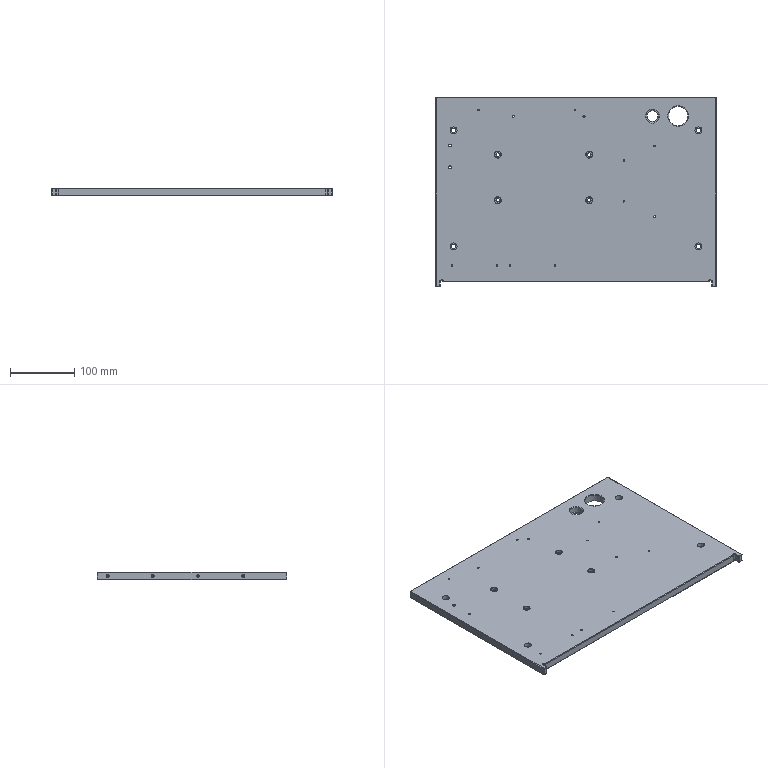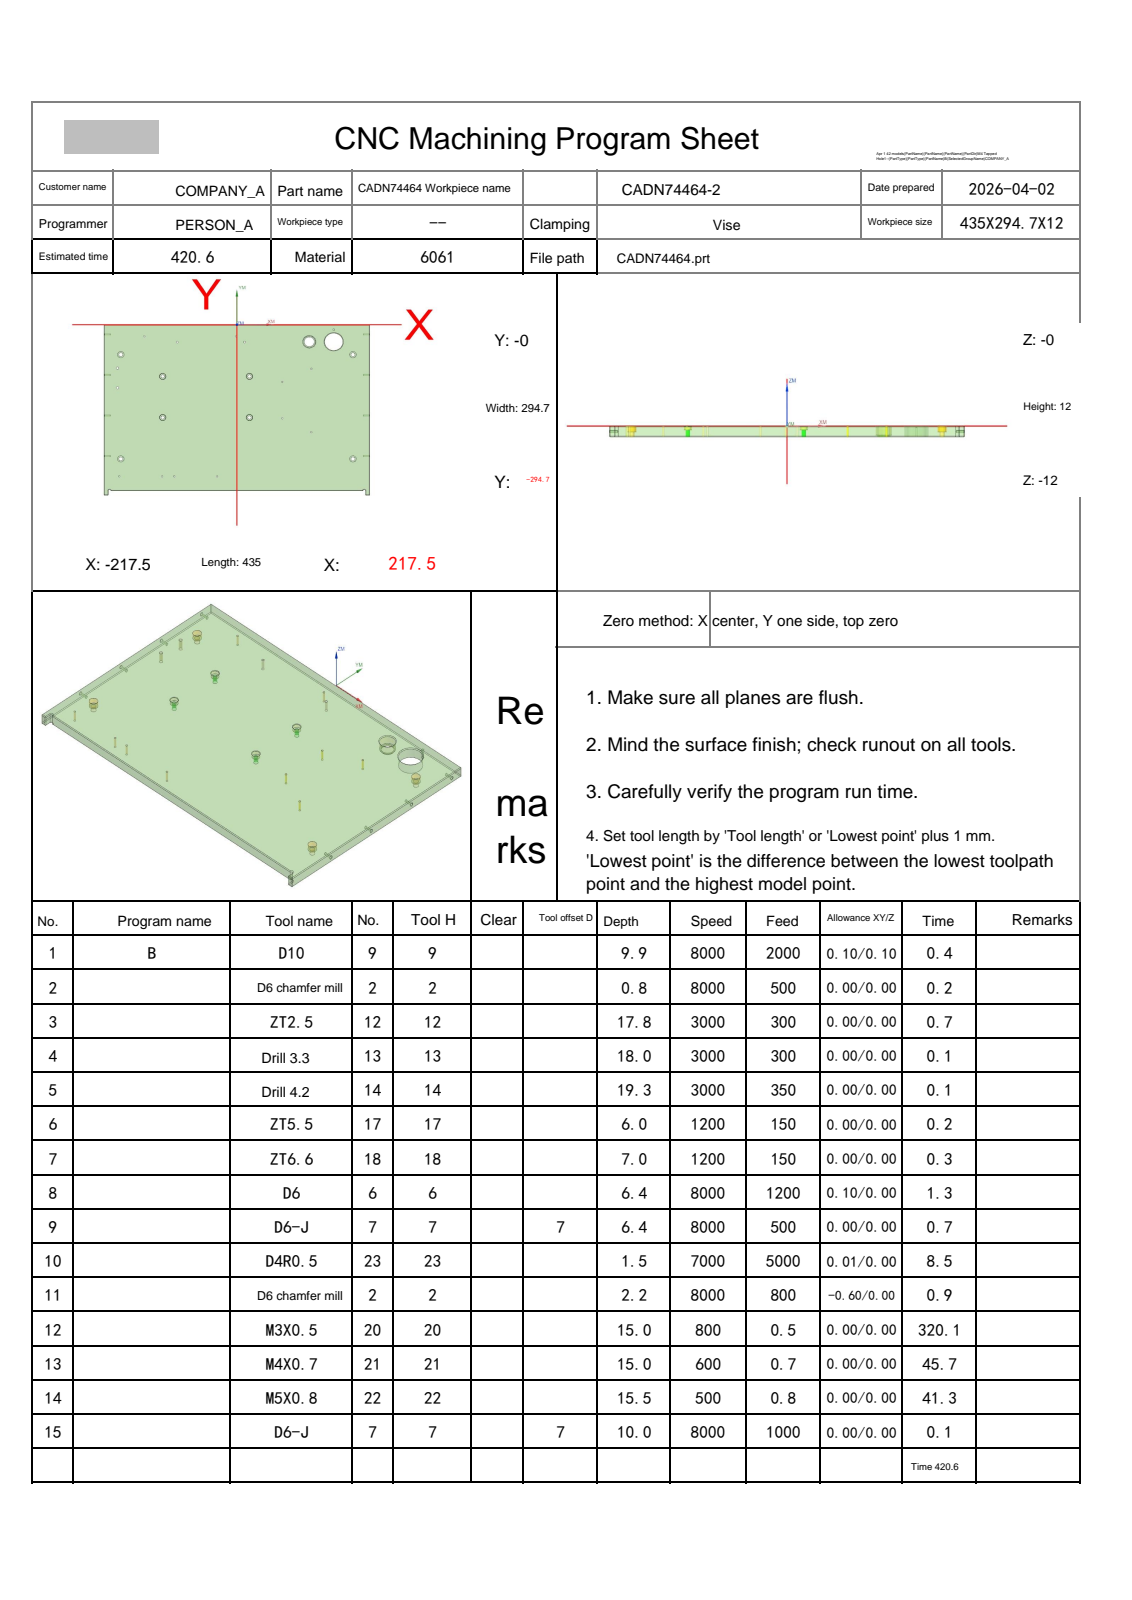NC program | NX | posted by the shop | part box 435 x 294.7 x 12 mm
Lines 33526 to 33933 of 33933:
N11 T02 M06
(D6 chamfer mill  D=6. R=0. H=02 ce=0.00 di=0.00)
G00 G90 G54 X-151.5 Y-20. M03 S8000
G43 H02 Z20.
M08
G98 G81 X-151.5 Y-20. Z-1.75 R3. F500.
X-1.5
X74.218 Y-98.649
X121.901 Y-76.021
Y-185.521
X74.218 Y-161.649
X-32.5 Y-261.7
X-102.5
X-122.5
X-192.5
G80
G00 Z20.
G00 G90 X-97.5 Y-30. M03 S8000
Z20.
G98 G81 X-97.5 Y-30. Z-2.2 R3. F500.
X12.5
G80
G00 Z20.
G00 G90 X-195.593 Y-108.306 M03 S8000
Z20.
Z-.5
G01 Z-1. F500.
X-195.7 Y-107.5
G03 X-197.2 Y-109. I0.0 J-1.5
X-195.5 Y-110.7 I1.7 J0.0
X-193.8 Y-109. I0.0 J1.7
X-195.5 Y-107.3 I-1.7 J0.0
X-197.2 Y-109. I0.0 J-1.7
X-195.7 Y-110.5 I1.5 J0.0
G01 X-195.593 Y-109.694
Z-.5
G00 Z20.
Y-74.306
Z-.5
G01 Z-1.
X-195.7 Y-73.5
G03 X-197.2 Y-75. I0.0 J-1.5
X-195.5 Y-76.7 I1.7 J0.0
X-193.8 Y-75. I0.0 J1.7
X-195.5 Y-73.3 I-1.7 J0.0
X-197.2 Y-75. I0.0 J-1.7
X-195.7 Y-76.5 I1.5 J0.0
G01 X-195.593 Y-75.694
Z-.5
G00 Z20.
G00 G90 X-125.117 Y-161.779 M03 S8000
Z20.
Z2.5
G01 X-124.98 Y-162.081 Z2.379 F800.
X-124.765 Y-162.447 Z2.225
X-124.512 Y-162.789 Z2.07
X-124.225 Y-163.102 Z1.916
X-123.906 Y-163.382 Z1.761
X-123.559 Y-163.627 Z1.606
X-123.291 Y-163.782 Z1.494
X-122.905 Y-163.96 Z1.339
X-122.503 Y-164.096 Z1.184
X-122.088 Y-164.188 Z1.03
X-121.666 Y-164.237 Z.875
X-121.241 Y-164.24 Z.721
X-120.819 Y-164.198 Z.566
X-120.403 Y-164.111 Z.412
X-119.999 Y-163.981 Z.257
X-119.61 Y-163.809 Z.102
X-119.243 Y-163.596 Z-.052
X-118.899 Y-163.346 Z-.207
X-118.584 Y-163.061 Z-.361
X-118.302 Y-162.744 Z-.516
X-118.054 Y-162.399 Z-.671
X-117.844 Y-162.03 Z-.825
X-117.675 Y-161.64 Z-.98
X-117.548 Y-161.235 Z-1.134
X-117.464 Y-160.819 Z-1.289
X-117.425 Y-160.396 Z-1.444
Y-160.241 Z-1.5
G03 X-121.425 Y-156.241 I-4. J0.0
X-125.425 Y-160.241 I0.0 J-4.
X-121.425 Y-164.241 I4. J0.0
X-117.425 Y-160.241 I0.0 J4.
X-117.456 Y-159.742 I-4. J0.0
G01 Z1.
G00 Z20.
X-125.117 Y-90.779
Z2.5
G01 X-124.98 Y-91.081 Z2.379
X-124.765 Y-91.447 Z2.225
X-124.512 Y-91.789 Z2.07
X-124.225 Y-92.102 Z1.916
X-123.906 Y-92.382 Z1.761
X-123.559 Y-92.627 Z1.606
X-123.291 Y-92.782 Z1.494
X-122.905 Y-92.96 Z1.339
X-122.503 Y-93.096 Z1.184
X-122.088 Y-93.188 Z1.03
X-121.666 Y-93.237 Z.875
X-121.241 Y-93.24 Z.721
X-120.819 Y-93.198 Z.566
X-120.403 Y-93.111 Z.412
X-119.999 Y-92.981 Z.257
X-119.61 Y-92.809 Z.102
X-119.243 Y-92.596 Z-.052
X-118.899 Y-92.346 Z-.207
X-118.584 Y-92.061 Z-.361
X-118.302 Y-91.744 Z-.516
X-118.054 Y-91.399 Z-.671
X-117.844 Y-91.03 Z-.825
X-117.675 Y-90.64 Z-.98
X-117.548 Y-90.235 Z-1.134
X-117.464 Y-89.819 Z-1.289
X-117.425 Y-89.396 Z-1.444
Y-89.241 Z-1.5
G03 X-121.425 Y-85.241 I-4. J0.0
X-125.425 Y-89.241 I0.0 J-4.
X-121.425 Y-93.241 I4. J0.0
X-117.425 Y-89.241 I0.0 J4.
X-117.456 Y-88.742 I-4. J0.0
G01 Z1.
G00 Z20.
X16.883 Y-90.779
Z2.5
G01 X17.02 Y-91.081 Z2.379
X17.235 Y-91.447 Z2.225
X17.488 Y-91.789 Z2.07
X17.775 Y-92.102 Z1.916
X18.094 Y-92.382 Z1.761
X18.441 Y-92.627 Z1.606
X18.709 Y-92.782 Z1.494
X19.095 Y-92.96 Z1.339
X19.497 Y-93.096 Z1.184
X19.912 Y-93.188 Z1.03
X20.334 Y-93.237 Z.875
X20.759 Y-93.24 Z.721
X21.181 Y-93.198 Z.566
X21.597 Y-93.111 Z.412
X22.001 Y-92.981 Z.257
X22.39 Y-92.809 Z.102
X22.757 Y-92.596 Z-.052
X23.101 Y-92.346 Z-.207
X23.416 Y-92.061 Z-.361
X23.698 Y-91.744 Z-.516
X23.946 Y-91.399 Z-.671
X24.156 Y-91.03 Z-.825
X24.325 Y-90.64 Z-.98
X24.452 Y-90.235 Z-1.134
X24.536 Y-89.819 Z-1.289
X24.575 Y-89.396 Z-1.444
Y-89.241 Z-1.5
G03 X20.575 Y-85.241 I-4. J0.0
X16.575 Y-89.241 I0.0 J-4.
X20.575 Y-93.241 I4. J0.0
X24.575 Y-89.241 I0.0 J4.
X24.544 Y-88.742 I-4. J0.0
G01 Z1.
G00 Z20.
X16.883 Y-161.779
Z2.5
G01 X17.02 Y-162.081 Z2.379
X17.235 Y-162.447 Z2.225
X17.488 Y-162.789 Z2.07
X17.775 Y-163.102 Z1.916
X18.094 Y-163.382 Z1.761
X18.441 Y-163.627 Z1.606
X18.709 Y-163.782 Z1.494
X19.095 Y-163.96 Z1.339
X19.497 Y-164.096 Z1.184
X19.912 Y-164.188 Z1.03
X20.334 Y-164.237 Z.875
X20.759 Y-164.24 Z.721
X21.181 Y-164.198 Z.566
X21.597 Y-164.111 Z.412
X22.001 Y-163.981 Z.257
X22.39 Y-163.809 Z.102
X22.757 Y-163.596 Z-.052
X23.101 Y-163.346 Z-.207
X23.416 Y-163.061 Z-.361
X23.698 Y-162.744 Z-.516
X23.946 Y-162.399 Z-.671
X24.156 Y-162.03 Z-.825
X24.325 Y-161.64 Z-.98
X24.452 Y-161.235 Z-1.134
X24.536 Y-160.819 Z-1.289
X24.575 Y-160.396 Z-1.444
Y-160.241 Z-1.5
G03 X20.575 Y-156.241 I-4. J0.0
X16.575 Y-160.241 I0.0 J-4.
X20.575 Y-164.241 I4. J0.0
X24.575 Y-160.241 I0.0 J4.
X24.544 Y-159.742 I-4. J0.0
G01 Z1.
G00 Z20.
G00 G90 X187.991 Y-236.053 M03 S8000
Z20.
Z2.5
G01 X188.166 Y-236.135 Z2.43 F800.
X188.601 Y-236.291 Z2.261
X189.05 Y-236.404 Z2.093
X189.507 Y-236.474 Z1.925
X189.969 Y-236.499 Z1.756
X190.431 Y-236.48 Z1.588
X190.89 Y-236.416 Z1.419
X191.34 Y-236.309 Z1.251
X191.777 Y-236.158 Z1.083
X192.198 Y-235.967 Z.914
X192.599 Y-235.735 Z.746
X192.976 Y-235.466 Z.577
X193.325 Y-235.163 Z.409
X193.643 Y-234.827 Z.241
X193.927 Y-234.462 Z.072
X194.175 Y-234.071 Z-.096
X194.384 Y-233.658 Z-.265
X194.552 Y-233.227 Z-.433
X194.679 Y-232.782 Z-.601
X194.761 Y-232.327 Z-.77
X194.8 Y-231.866 Z-.938
Y-231.696 Z-1.
G03 X190. Y-226.896 I-4.8 J0.0
X185.2 Y-231.696 I0.0 J-4.8
X190. Y-236.496 I4.8 J0.0
X194.8 Y-231.696 I0.0 J4.8
X194.774 Y-231.197 I-4.8 J0.0
G01 Z1.5
G00 Z20.
X187.991 Y-56.053
Z2.5
G01 X188.166 Y-56.135 Z2.43
X188.601 Y-56.291 Z2.261
X189.05 Y-56.404 Z2.093
X189.507 Y-56.474 Z1.925
X189.969 Y-56.499 Z1.756
X190.431 Y-56.48 Z1.588
X190.89 Y-56.416 Z1.419
X191.34 Y-56.309 Z1.251
X191.777 Y-56.158 Z1.083
X192.198 Y-55.967 Z.914
X192.599 Y-55.735 Z.746
X192.976 Y-55.466 Z.577
X193.325 Y-55.163 Z.409
X193.643 Y-54.827 Z.241
X193.927 Y-54.462 Z.072
X194.175 Y-54.071 Z-.096
X194.384 Y-53.658 Z-.265
X194.552 Y-53.227 Z-.433
X194.679 Y-52.782 Z-.601
X194.761 Y-52.327 Z-.77
X194.8 Y-51.866 Z-.938
Y-51.696 Z-1.
G03 X190. Y-46.896 I-4.8 J0.0
X185.2 Y-51.696 I0.0 J-4.8
X190. Y-56.496 I4.8 J0.0
X194.8 Y-51.696 I0.0 J4.8
X194.774 Y-51.197 I-4.8 J0.0
G01 Z1.5
G00 Z20.
X-192.009 Y-56.053
Z2.5
G01 X-191.834 Y-56.135 Z2.43
X-191.399 Y-56.291 Z2.261
X-190.95 Y-56.404 Z2.093
X-190.493 Y-56.474 Z1.925
X-190.031 Y-56.499 Z1.756
X-189.569 Y-56.48 Z1.588
X-189.11 Y-56.416 Z1.419
X-188.66 Y-56.309 Z1.251
X-188.223 Y-56.158 Z1.083
X-187.802 Y-55.967 Z.914
X-187.401 Y-55.735 Z.746
X-187.024 Y-55.466 Z.577
X-186.675 Y-55.163 Z.409
X-186.357 Y-54.827 Z.241
X-186.073 Y-54.462 Z.072
X-185.825 Y-54.071 Z-.096
X-185.616 Y-53.658 Z-.265
X-185.448 Y-53.227 Z-.433
X-185.321 Y-52.782 Z-.601
X-185.239 Y-52.327 Z-.77
X-185.2 Y-51.866 Z-.938
Y-51.696 Z-1.
G03 X-190. Y-46.896 I-4.8 J0.0
X-194.8 Y-51.696 I0.0 J-4.8
X-190. Y-56.496 I4.8 J0.0
X-185.2 Y-51.696 I0.0 J4.8
X-185.226 Y-51.197 I-4.8 J0.0
G01 Z1.5
G00 Z20.
X-192.009 Y-236.053
Z2.5
G01 X-191.834 Y-236.135 Z2.43
X-191.399 Y-236.291 Z2.261
X-190.95 Y-236.404 Z2.093
X-190.493 Y-236.474 Z1.925
X-190.031 Y-236.499 Z1.756
X-189.569 Y-236.48 Z1.588
X-189.11 Y-236.416 Z1.419
X-188.66 Y-236.309 Z1.251
X-188.223 Y-236.158 Z1.083
X-187.802 Y-235.967 Z.914
X-187.401 Y-235.735 Z.746
X-187.024 Y-235.466 Z.577
X-186.675 Y-235.163 Z.409
X-186.357 Y-234.827 Z.241
X-186.073 Y-234.462 Z.072
X-185.825 Y-234.071 Z-.096
X-185.616 Y-233.658 Z-.265
X-185.448 Y-233.227 Z-.433
X-185.321 Y-232.782 Z-.601
X-185.239 Y-232.327 Z-.77
X-185.2 Y-231.866 Z-.938
Y-231.696 Z-1.
G03 X-190. Y-226.896 I-4.8 J0.0
X-194.8 Y-231.696 I0.0 J-4.8
X-190. Y-236.496 I4.8 J0.0
X-185.2 Y-231.696 I0.0 J4.8
X-185.226 Y-231.197 I-4.8 J0.0
G01 Z1.5
G00 Z20.
G91 G28 Z0.0
M05
M09
G91 G28 Z0.0
M01
N12 T20 M06
(M3X0.5 D=2.5 DR_a=180 H=20)
G00 G90 G54 X-151.5 Y-20. M03 S800
G43 H20 Z20.
M08
G95
G98 G84 X-151.5 Y-20. Z-15. R1. F.5 Q5.
X-1.5
G98 G84 X74.218 Y-98.649 Z-15. R1.
X121.901 Y-76.021
Y-185.521
X74.218 Y-161.649
G98 G84 X-32.5 Y-261.7 Z-15. R1.
X-102.5
X-122.5
X-192.5
G80
G94
G00 Z20.
G91 G28 Z0.0
M05
M09
G91 G28 Z0.0
M01
N13 T21 M06
(M4X0.7 D=3.3 DR_a=180 H=21)
G00 G90 G54 X-97.5 Y-30. M03 S600
G43 H21 Z20.
M08
G95
G98 G84 X-97.5 Y-30. Z-15. R1. F.7 Q4.
X12.5
G80
G94
G00 Z20.
G91 G28 Z0.0
M05
M09
G91 G28 Z0.0
M01
N14 T22 M06
(M5X0.8 D=4.2 DR_a=180 H=22)
G00 G90 G54 X-195.5 Y-109. M03 S500
G43 H22 Z20.
M08
G95
G98 G84 X-195.5 Y-109. Z-15.5 R1. F.8 Q3.
Y-75.
G80
G94
G00 Z20.
G91 G28 Z0.0
M05
M09
G91 G28 Z0.0
M01
N15 T07 M06
(D6-J  D=6. R=0. H=07 ce=0.00 di=0.00)
G00 G90 G54 X119.4 Y-23.667 M03 S8000
G43 H07 Z10.
M08
Z-8.5
G01 Z-10. F1000.
G41 D07
Y-23.4
G03 X118.5 Y-22.5 I-.9 J0.0
X111.5 Y-29.5 I0.0 J-7.
X118.5 Y-36.5 I7. J0.0
X125.5 Y-29.5 I0.0 J7.
X118.5 Y-22.5 I-7. J0.0
X118.1 Y-22.511 I0.0 J-7.
X117.252 Y-23.41 I.051 J-.899
G01 X117.253 Y-23.461
X117.257 Y-23.528
G40 X117.268 Y-23.728
Z-8.5
G00 Z10.
M05
M09
G91 G28 Z0.0
G91 G28 Y0.0
M30
%